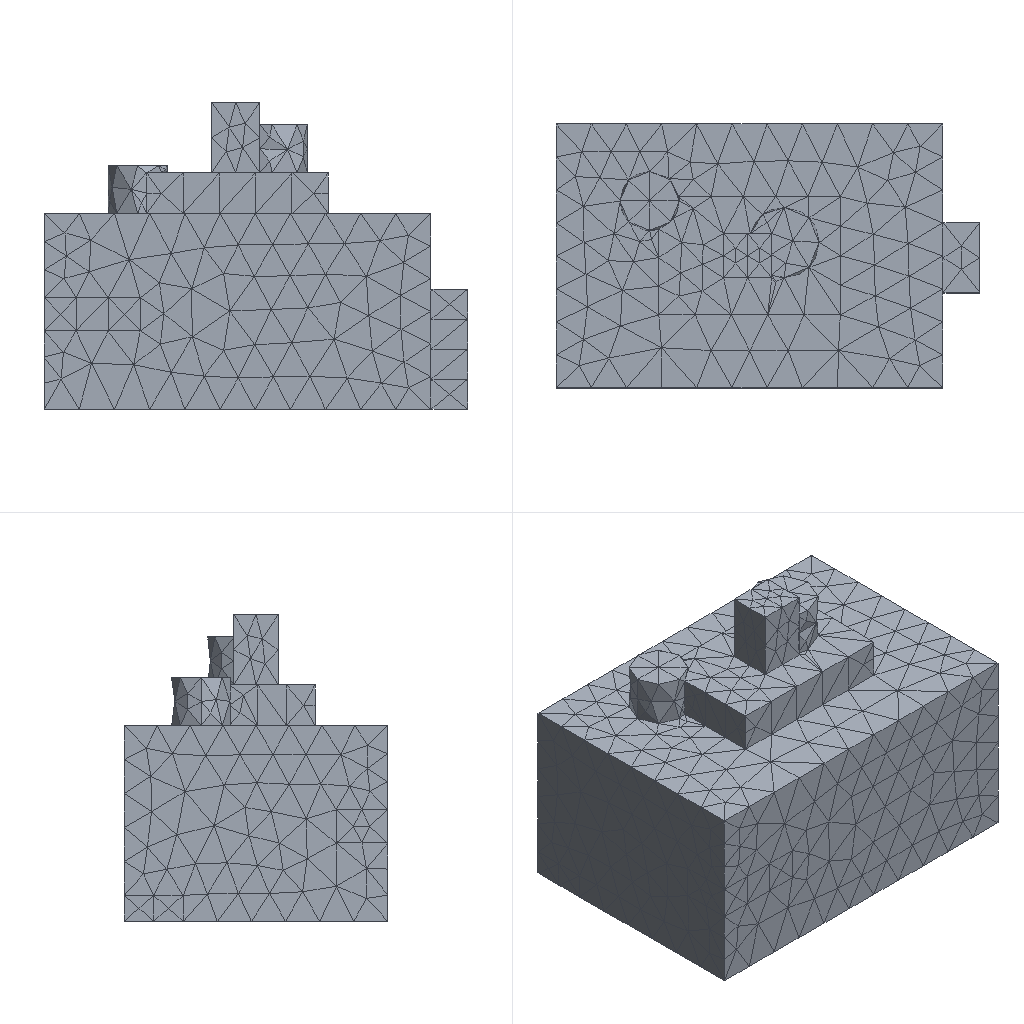Simulation study | ansys mapdl
Set-up summary:
category,name,step,type,value,unit,region
solver,ansys_mapdl
units,mm-N-s-tonne (MPa),,inferred,E=210000 density=
analysis,model,,static
mesh,nodes,,,8770
mesh,elements,,,5617
element_type,SOLID187,,,5617
material,mat 1,,E,210000
material,mat 1,,nu,0.3
load,,model,body load temp,,,all
load,,model,force,"1000 [dir=(0, 0, -1) n=386]",,node list
bc,,model,fixed,"[dofs=UX,UY,UZ n=8624]",,node list
Ansys APDL input file, long lists of numbers shortened:
/COM,ANSYS RELEASE 2026 R1           BUILD 26.1      UP20260202       09:10:32
/PREP7
/NOPR
/TITLE,2
ANTYPE, 0
*IF,_CDRDOFF,EQ,1,THEN     !if solid model was read in
_CDRDOFF=             !reset flag, numoffs already performed
*ELSE              !offset database for the following FE model
NUMOFF,NODE,     8770
NUMOFF,ELEM,     5617
NUMOFF,MAT ,        1
NUMOFF,TYPE,        1
*ENDIF
*SET,_RETURN ,  0.
*SET,_STATUS ,  0.
*SET,_UIQR   ,  386.
*SET,__FLOATPARAMETER__,  8770.
DOF,DELETE
ETBLOCK,        1,        1
(2i9,19a9)
        1      187        0        0        0        0        0        0        0        0        0        0        0        0        0        0        0        0        0        0        0
       -1
NBLOCK,6,SOLID,      8770,      8770
(3i9,6e21.13e3)
        1        0        0 6.0000000000000E+000 6.0000000000000E+000 8.2980000000000E+001
! (8769 more lines like these left out)
N,UNBL,LOC,       -1,
EBLOCK,19,SOLID,      5617,      5617
(19i10)
         1         1         1         1         0         0         0         0        10         0         1      2475      2476      2477      2478      3123      3124      3125      3126
! (11233 more lines like these left out)
        -1
MPTEMP,UNBL, 1, 1,  0.    ,
MPDATA,UNBL, 1,EX  ,       1, 1,  210000.000    ,
MPTEMP,UNBL, 1, 1,  0.    ,
MPDATA,UNBL, 1,NUXY,       1, 1, 0.3    ,
MPTEMP,UNBL, 1, 1,  0.    ,
MPDATA,UNBL, 1,PRXY,       1, 1, 0.3    ,
EXTOPT,ATTR,      0,      0,      0
EXTOPT,ESIZE,  0,  0.
EXTOPT,ACLEAR,      0
TREF,  0.
IRLF,  0
BFUNIF,TEMP,_TINY
ACEL,  0.    ,  0.    ,  0.
OMEGA,  0.    ,  0.    ,  0.
DOMEGA,  0.    ,  0.    ,  0.
CGLOC,  0.    ,  0.    ,  0.
CGOMEGA,  0.    ,  0.    ,  0.
DCGOMG,  0.    ,  0.    ,  0.
KUSE,     0
TIME,  0.
ALPHAD,  0.
BETAD,  0.
DMPRAT,  0.
DMPSTR,  0.
CRPLIM, 0.1    ,   0
CRPLIM,  0.    ,   1
NCNV,     0, 1.000000000E+12,     0,  0.    ,  0.
NEQIT,     0
ERESX,DEFA
DBLOCK,      8624
(i9,a6,2(pg16.9))
      407  UX    0.00000000      0.00000000
! (8623 more lines like these left out)
       -1
FBLOCK,       386
(i9,a6,2(pg16.9))
        1  FZ   -2.59067358      0.00000000
! (385 more lines like these left out)
       -1
/GO
FINISH
Results summary:
result,analysis_type_db,,,static,unstated
result,n_sets,,,1,unstated
result,load_steps[0].set,load_step=1,,1,unstated
result,load_steps[0].substep,load_step=1,,1,unstated
result,load_steps[0].time,load_step=1,,1,unstated
result,load_steps[0].freq,load_step=1,,1,unstated
result,load_steps[0].max_usum,load_step=1,,0.0004403,unstated
result,load_steps[0].max_seqv,load_step=1,,4.413,unstated
result,load_steps[0].reaction_sum.FX,load_step=1,,4.089e-11,unstated
result,load_steps[0].reaction_sum.FY,load_step=1,,-3.37508e-12,unstated
result,load_steps[0].reaction_sum.FZ,load_step=1,,1000,unstated
result,load_steps[0].reaction_sum.MX,load_step=1,,0,unstated
result,load_steps[0].reaction_sum.MY,load_step=1,,0,unstated
result,load_steps[0].reaction_sum.MZ,load_step=1,,0,unstated
result,convergence,,,results present for all listed sets,unstated